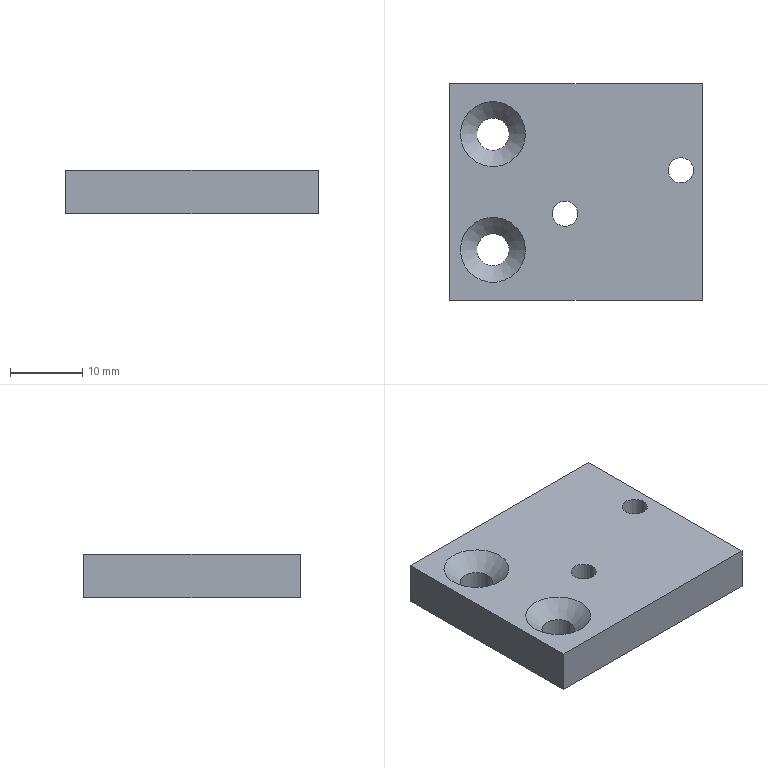Part | NX | 1 solid | 14 faces | box 35 x 30 x 6 mm | volume 5854 mm3 | plane 6 | cylinder 4 | cone 4 | commonest cylinder face diameters 3.5 x2 4.5 x2
STEP:
#1=CARTESIAN_POINT('',(17.5,-15.,0.));
#2=VERTEX_POINT('',#1);
#3=CARTESIAN_POINT('',(17.5,1.197,0.));
#4=VERTEX_POINT('',#3);
#5=CARTESIAN_POINT('',(17.5,-15.,0.));
#6=DIRECTION('',(0.,1.,0.));
#7=VECTOR('',#6,1000.);
#8=LINE('',#5,#7);
#9=EDGE_CURVE('',#2,#4,#8,.T.);
#10=ORIENTED_EDGE('',*,*,#9,.T.);
#11=CARTESIAN_POINT('',(17.5,4.803,0.));
#12=VERTEX_POINT('',#11);
#13=CARTESIAN_POINT('',(17.5,1.197,0.));
#14=CARTESIAN_POINT('',(17.5,1.756,0.2876));
#15=CARTESIAN_POINT('',(17.5,2.993,0.7128));
#16=CARTESIAN_POINT('',(17.5,4.246,0.2868));
#17=CARTESIAN_POINT('',(17.5,4.803,0.));
#18=B_SPLINE_CURVE_WITH_KNOTS('',3,(#13,#14,#15,#16,#17),.UNSPECIFIED.,.F.,.F.,(4,1,4),(0.004834,0.006713,0.008592),.UNSPECIFIED.);
#19=EDGE_CURVE('',#4,#12,#18,.T.);
#20=ORIENTED_EDGE('',*,*,#19,.T.);
#21=CARTESIAN_POINT('',(17.5,15.,0.));
#22=VERTEX_POINT('',#21);
#23=CARTESIAN_POINT('',(17.5,-15.,0.));
#24=DIRECTION('',(0.,1.,0.));
#25=VECTOR('',#24,1000.);
#26=LINE('',#23,#25);
#27=EDGE_CURVE('',#12,#22,#26,.T.);
#28=ORIENTED_EDGE('',*,*,#27,.T.);
#29=CARTESIAN_POINT('',(17.5,15.,6.));
#30=VERTEX_POINT('',#29);
#31=CARTESIAN_POINT('',(17.5,15.,6.));
#32=DIRECTION('',(0.,0.,-1.));
#33=VECTOR('',#32,1000.);
#34=LINE('',#31,#33);
#35=EDGE_CURVE('',#30,#22,#34,.T.);
#36=ORIENTED_EDGE('',*,*,#35,.F.);
#37=CARTESIAN_POINT('',(17.5,-15.,6.));
#38=VERTEX_POINT('',#37);
#39=CARTESIAN_POINT('',(17.5,-15.,6.));
#40=DIRECTION('',(0.,1.,0.));
#41=VECTOR('',#40,1000.);
#42=LINE('',#39,#41);
#43=EDGE_CURVE('',#38,#30,#42,.T.);
#44=ORIENTED_EDGE('',*,*,#43,.F.);
#45=CARTESIAN_POINT('',(17.5,-15.,6.));
#46=DIRECTION('',(0.,0.,-1.));
#47=VECTOR('',#46,1000.);
#48=LINE('',#45,#47);
#49=EDGE_CURVE('',#38,#2,#48,.T.);
#50=ORIENTED_EDGE('',*,*,#49,.T.);
#51=EDGE_LOOP('',(#10,#20,#28,#36,#44,#50));
#52=FACE_BOUND('',#51,.T.);
#53=CARTESIAN_POINT('',(17.5,-15.,6.));
#54=DIRECTION('',(-1.,0.,0.));
#55=DIRECTION('',(0.,0.,1.));
#56=AXIS2_PLACEMENT_3D('',#53,#54,#55);
#57=PLANE('',#56);
#58=ADVANCED_FACE('',(#52),#57,.F.);
#59=CARTESIAN_POINT('',(-17.5,15.,0.));
#60=VERTEX_POINT('',#59);
#61=CARTESIAN_POINT('',(-17.5,15.,0.));
#62=DIRECTION('',(-1.,0.,0.));
#63=VECTOR('',#62,1000.);
#64=LINE('',#61,#63);
#65=EDGE_CURVE('',#22,#60,#64,.T.);
#66=ORIENTED_EDGE('',*,*,#65,.T.);
#67=CARTESIAN_POINT('',(-17.5,15.,6.));
#68=VERTEX_POINT('',#67);
#69=CARTESIAN_POINT('',(-17.5,15.,6.));
#70=DIRECTION('',(0.,0.,-1.));
#71=VECTOR('',#70,1000.);
#72=LINE('',#69,#71);
#73=EDGE_CURVE('',#68,#60,#72,.T.);
#74=ORIENTED_EDGE('',*,*,#73,.F.);
#75=CARTESIAN_POINT('',(-17.5,15.,6.));
#76=DIRECTION('',(-1.,0.,0.));
#77=VECTOR('',#76,1000.);
#78=LINE('',#75,#77);
#79=EDGE_CURVE('',#30,#68,#78,.T.);
#80=ORIENTED_EDGE('',*,*,#79,.F.);
#81=ORIENTED_EDGE('',*,*,#35,.T.);
#82=EDGE_LOOP('',(#66,#74,#80,#81));
#83=FACE_BOUND('',#82,.T.);
#84=CARTESIAN_POINT('',(-17.5,15.,6.));
#85=DIRECTION('',(0.,-1.,0.));
#86=DIRECTION('',(0.,0.,-1.));
#87=AXIS2_PLACEMENT_3D('',#84,#85,#86);
#88=PLANE('',#87);
#89=ADVANCED_FACE('',(#83),#88,.F.);
#90=CARTESIAN_POINT('',(-17.5,-15.,0.));
#91=VERTEX_POINT('',#90);
#92=CARTESIAN_POINT('',(-17.5,-15.,0.));
#93=DIRECTION('',(0.,-1.,0.));
#94=VECTOR('',#93,1000.);
#95=LINE('',#92,#94);
#96=EDGE_CURVE('',#60,#91,#95,.T.);
#97=ORIENTED_EDGE('',*,*,#96,.T.);
#98=CARTESIAN_POINT('',(-17.5,-15.,6.));
#99=VERTEX_POINT('',#98);
#100=CARTESIAN_POINT('',(-17.5,-15.,6.));
#101=DIRECTION('',(0.,0.,-1.));
#102=VECTOR('',#101,1000.);
#103=LINE('',#100,#102);
#104=EDGE_CURVE('',#99,#91,#103,.T.);
#105=ORIENTED_EDGE('',*,*,#104,.F.);
#106=CARTESIAN_POINT('',(-17.5,-15.,6.));
#107=DIRECTION('',(0.,-1.,0.));
#108=VECTOR('',#107,1000.);
#109=LINE('',#106,#108);
#110=EDGE_CURVE('',#68,#99,#109,.T.);
#111=ORIENTED_EDGE('',*,*,#110,.F.);
#112=ORIENTED_EDGE('',*,*,#73,.T.);
#113=EDGE_LOOP('',(#97,#105,#111,#112));
#114=FACE_BOUND('',#113,.T.);
#115=CARTESIAN_POINT('',(-17.5,-15.,6.));
#116=DIRECTION('',(1.,0.,0.));
#117=DIRECTION('',(0.,0.,-1.));
#118=AXIS2_PLACEMENT_3D('',#115,#116,#117);
#119=PLANE('',#118);
#120=ADVANCED_FACE('',(#114),#119,.F.);
#121=CARTESIAN_POINT('',(-17.5,-15.,0.));
#122=DIRECTION('',(1.,0.,0.));
#123=VECTOR('',#122,1000.);
#124=LINE('',#121,#123);
#125=EDGE_CURVE('',#91,#2,#124,.T.);
#126=ORIENTED_EDGE('',*,*,#125,.T.);
#127=ORIENTED_EDGE('',*,*,#49,.F.);
#128=CARTESIAN_POINT('',(-17.5,-15.,6.));
#129=DIRECTION('',(1.,0.,0.));
#130=VECTOR('',#129,1000.);
#131=LINE('',#128,#130);
#132=EDGE_CURVE('',#99,#38,#131,.T.);
#133=ORIENTED_EDGE('',*,*,#132,.F.);
#134=ORIENTED_EDGE('',*,*,#104,.T.);
#135=EDGE_LOOP('',(#126,#127,#133,#134));
#136=FACE_BOUND('',#135,.T.);
#137=CARTESIAN_POINT('',(-17.5,-15.,6.));
#138=DIRECTION('',(0.,1.,0.));
#139=DIRECTION('',(0.,0.,1.));
#140=AXIS2_PLACEMENT_3D('',#137,#138,#139);
#141=PLANE('',#140);
#142=ADVANCED_FACE('',(#136),#141,.F.);
#143=CARTESIAN_POINT('',(-3.25,-3.,6.));
#144=VERTEX_POINT('',#143);
#145=CARTESIAN_POINT('',(-1.5,-3.,6.));
#146=DIRECTION('',(0.,0.,-1.));
#147=DIRECTION('',(-1.,0.,0.));
#148=AXIS2_PLACEMENT_3D('',#145,#146,#147);
#149=CIRCLE('',#148,1.75);
#150=EDGE_CURVE('',#144,#144,#149,.T.);
#151=ORIENTED_EDGE('',*,*,#150,.T.);
#152=EDGE_LOOP('',(#151));
#153=FACE_BOUND('',#152,.T.);
#154=CARTESIAN_POINT('',(12.75,3.,6.));
#155=VERTEX_POINT('',#154);
#156=CARTESIAN_POINT('',(14.5,3.,6.));
#157=DIRECTION('',(0.,0.,-1.));
#158=DIRECTION('',(-1.,0.,0.));
#159=AXIS2_PLACEMENT_3D('',#156,#157,#158);
#160=CIRCLE('',#159,1.75);
#161=EDGE_CURVE('',#155,#155,#160,.T.);
#162=ORIENTED_EDGE('',*,*,#161,.T.);
#163=EDGE_LOOP('',(#162));
#164=FACE_BOUND('',#163,.T.);
#165=CARTESIAN_POINT('',(-7.,8.,6.));
#166=VERTEX_POINT('',#165);
#167=CARTESIAN_POINT('',(-11.5,8.,6.));
#168=DIRECTION('',(0.,0.,1.));
#169=DIRECTION('',(1.,0.,0.));
#170=AXIS2_PLACEMENT_3D('',#167,#168,#169);
#171=CIRCLE('',#170,4.5);
#172=EDGE_CURVE('',#166,#166,#171,.T.);
#173=ORIENTED_EDGE('',*,*,#172,.F.);
#174=EDGE_LOOP('',(#173));
#175=FACE_BOUND('',#174,.T.);
#176=CARTESIAN_POINT('',(-7.,-8.,6.));
#177=VERTEX_POINT('',#176);
#178=CARTESIAN_POINT('',(-11.5,-8.,6.));
#179=DIRECTION('',(0.,0.,1.));
#180=DIRECTION('',(1.,0.,0.));
#181=AXIS2_PLACEMENT_3D('',#178,#179,#180);
#182=CIRCLE('',#181,4.5);
#183=EDGE_CURVE('',#177,#177,#182,.T.);
#184=ORIENTED_EDGE('',*,*,#183,.F.);
#185=EDGE_LOOP('',(#184));
#186=FACE_BOUND('',#185,.T.);
#187=ORIENTED_EDGE('',*,*,#43,.T.);
#188=ORIENTED_EDGE('',*,*,#79,.T.);
#189=ORIENTED_EDGE('',*,*,#110,.T.);
#190=ORIENTED_EDGE('',*,*,#132,.T.);
#191=EDGE_LOOP('',(#187,#188,#189,#190));
#192=FACE_BOUND('',#191,.T.);
#193=CARTESIAN_POINT('',(0.,0.,6.));
#194=DIRECTION('',(0.,0.,-1.));
#195=DIRECTION('',(-1.,0.,0.));
#196=AXIS2_PLACEMENT_3D('',#193,#194,#195);
#197=PLANE('',#196);
#198=ADVANCED_FACE('',(#153,#164,#175,#186,#192),#197,.F.);
#199=CARTESIAN_POINT('',(-5.,-3.,0.));
#200=VERTEX_POINT('',#199);
#201=CARTESIAN_POINT('',(-1.5,-3.,0.));
#202=DIRECTION('',(0.,0.,-1.));
#203=DIRECTION('',(-1.,0.,0.));
#204=AXIS2_PLACEMENT_3D('',#201,#202,#203);
#205=CIRCLE('',#204,3.5);
#206=EDGE_CURVE('',#200,#200,#205,.T.);
#207=ORIENTED_EDGE('',*,*,#206,.F.);
#208=EDGE_LOOP('',(#207));
#209=FACE_BOUND('',#208,.T.);
#210=CARTESIAN_POINT('',(14.5,3.,0.));
#211=DIRECTION('',(0.,0.,-1.));
#212=DIRECTION('',(-1.,0.,0.));
#213=AXIS2_PLACEMENT_3D('',#210,#211,#212);
#214=CIRCLE('',#213,3.5);
#215=EDGE_CURVE('',#4,#12,#214,.T.);
#216=ORIENTED_EDGE('',*,*,#215,.F.);
#217=ORIENTED_EDGE('',*,*,#9,.F.);
#218=ORIENTED_EDGE('',*,*,#125,.F.);
#219=ORIENTED_EDGE('',*,*,#96,.F.);
#220=ORIENTED_EDGE('',*,*,#65,.F.);
#221=ORIENTED_EDGE('',*,*,#27,.F.);
#222=EDGE_LOOP('',(#216,#217,#218,#219,#220,#221));
#223=FACE_BOUND('',#222,.T.);
#224=CARTESIAN_POINT('',(-9.25,8.,0.));
#225=VERTEX_POINT('',#224);
#226=CARTESIAN_POINT('',(-11.5,8.,0.));
#227=DIRECTION('',(0.,0.,1.));
#228=DIRECTION('',(1.,0.,0.));
#229=AXIS2_PLACEMENT_3D('',#226,#227,#228);
#230=CIRCLE('',#229,2.25);
#231=EDGE_CURVE('',#225,#225,#230,.T.);
#232=ORIENTED_EDGE('',*,*,#231,.T.);
#233=EDGE_LOOP('',(#232));
#234=FACE_BOUND('',#233,.T.);
#235=CARTESIAN_POINT('',(-9.25,-8.,0.));
#236=VERTEX_POINT('',#235);
#237=CARTESIAN_POINT('',(-11.5,-8.,0.));
#238=DIRECTION('',(0.,0.,1.));
#239=DIRECTION('',(1.,0.,0.));
#240=AXIS2_PLACEMENT_3D('',#237,#238,#239);
#241=CIRCLE('',#240,2.25);
#242=EDGE_CURVE('',#236,#236,#241,.T.);
#243=ORIENTED_EDGE('',*,*,#242,.T.);
#244=EDGE_LOOP('',(#243));
#245=FACE_BOUND('',#244,.T.);
#246=CARTESIAN_POINT('',(0.,0.,0.));
#247=DIRECTION('',(0.,0.,-1.));
#248=DIRECTION('',(-1.,0.,0.));
#249=AXIS2_PLACEMENT_3D('',#246,#247,#248);
#250=PLANE('',#249);
#251=ADVANCED_FACE('',(#209,#223,#234,#245),#250,.T.);
#252=ORIENTED_EDGE('',*,*,#242,.F.);
#253=EDGE_LOOP('',(#252));
#254=FACE_BOUND('',#253,.T.);
#255=CARTESIAN_POINT('',(-9.25,-8.,3.75));
#256=VERTEX_POINT('',#255);
#257=CARTESIAN_POINT('',(-11.5,-8.,3.75));
#258=DIRECTION('',(0.,0.,1.));
#259=DIRECTION('',(1.,0.,0.));
#260=AXIS2_PLACEMENT_3D('',#257,#258,#259);
#261=CIRCLE('',#260,2.25);
#262=EDGE_CURVE('',#256,#256,#261,.T.);
#263=ORIENTED_EDGE('',*,*,#262,.T.);
#264=EDGE_LOOP('',(#263));
#265=FACE_BOUND('',#264,.T.);
#266=CARTESIAN_POINT('',(-11.5,-8.,6.));
#267=DIRECTION('',(0.,0.,1.));
#268=DIRECTION('',(1.,0.,0.));
#269=AXIS2_PLACEMENT_3D('',#266,#267,#268);
#270=CYLINDRICAL_SURFACE('',#269,2.25);
#271=ADVANCED_FACE('',(#254,#265),#270,.F.);
#272=ORIENTED_EDGE('',*,*,#262,.F.);
#273=EDGE_LOOP('',(#272));
#274=FACE_BOUND('',#273,.T.);
#275=ORIENTED_EDGE('',*,*,#183,.T.);
#276=EDGE_LOOP('',(#275));
#277=FACE_BOUND('',#276,.T.);
#278=CARTESIAN_POINT('',(-11.5,-8.,6.));
#279=DIRECTION('',(0.,0.,1.));
#280=DIRECTION('',(1.,0.,0.));
#281=AXIS2_PLACEMENT_3D('',#278,#279,#280);
#282=CONICAL_SURFACE('',#281,4.5,0.7854);
#283=ADVANCED_FACE('',(#274,#277),#282,.F.);
#284=ORIENTED_EDGE('',*,*,#231,.F.);
#285=EDGE_LOOP('',(#284));
#286=FACE_BOUND('',#285,.T.);
#287=CARTESIAN_POINT('',(-9.25,8.,3.75));
#288=VERTEX_POINT('',#287);
#289=CARTESIAN_POINT('',(-11.5,8.,3.75));
#290=DIRECTION('',(0.,0.,1.));
#291=DIRECTION('',(1.,0.,0.));
#292=AXIS2_PLACEMENT_3D('',#289,#290,#291);
#293=CIRCLE('',#292,2.25);
#294=EDGE_CURVE('',#288,#288,#293,.T.);
#295=ORIENTED_EDGE('',*,*,#294,.T.);
#296=EDGE_LOOP('',(#295));
#297=FACE_BOUND('',#296,.T.);
#298=CARTESIAN_POINT('',(-11.5,8.,6.));
#299=DIRECTION('',(0.,0.,1.));
#300=DIRECTION('',(1.,0.,0.));
#301=AXIS2_PLACEMENT_3D('',#298,#299,#300);
#302=CYLINDRICAL_SURFACE('',#301,2.25);
#303=ADVANCED_FACE('',(#286,#297),#302,.F.);
#304=ORIENTED_EDGE('',*,*,#294,.F.);
#305=EDGE_LOOP('',(#304));
#306=FACE_BOUND('',#305,.T.);
#307=ORIENTED_EDGE('',*,*,#172,.T.);
#308=EDGE_LOOP('',(#307));
#309=FACE_BOUND('',#308,.T.);
#310=CARTESIAN_POINT('',(-11.5,8.,6.));
#311=DIRECTION('',(0.,0.,1.));
#312=DIRECTION('',(1.,0.,0.));
#313=AXIS2_PLACEMENT_3D('',#310,#311,#312);
#314=CONICAL_SURFACE('',#313,4.5,0.7854);
#315=ADVANCED_FACE('',(#306,#309),#314,.F.);
#316=CARTESIAN_POINT('',(12.75,3.,1.75));
#317=VERTEX_POINT('',#316);
#318=CARTESIAN_POINT('',(14.5,3.,1.75));
#319=DIRECTION('',(0.,0.,-1.));
#320=DIRECTION('',(-1.,0.,0.));
#321=AXIS2_PLACEMENT_3D('',#318,#319,#320);
#322=CIRCLE('',#321,1.75);
#323=EDGE_CURVE('',#317,#317,#322,.T.);
#324=ORIENTED_EDGE('',*,*,#323,.F.);
#325=EDGE_LOOP('',(#324));
#326=FACE_BOUND('',#325,.T.);
#327=ORIENTED_EDGE('',*,*,#215,.T.);
#328=ORIENTED_EDGE('',*,*,#19,.F.);
#329=EDGE_LOOP('',(#327,#328));
#330=FACE_BOUND('',#329,.T.);
#331=CARTESIAN_POINT('',(14.5,3.,0.));
#332=DIRECTION('',(0.,0.,-1.));
#333=DIRECTION('',(-1.,0.,0.));
#334=AXIS2_PLACEMENT_3D('',#331,#332,#333);
#335=CONICAL_SURFACE('',#334,3.5,0.7854);
#336=ADVANCED_FACE('',(#326,#330),#335,.F.);
#337=ORIENTED_EDGE('',*,*,#161,.F.);
#338=EDGE_LOOP('',(#337));
#339=FACE_BOUND('',#338,.T.);
#340=ORIENTED_EDGE('',*,*,#323,.T.);
#341=EDGE_LOOP('',(#340));
#342=FACE_BOUND('',#341,.T.);
#343=CARTESIAN_POINT('',(14.5,3.,0.));
#344=DIRECTION('',(0.,0.,-1.));
#345=DIRECTION('',(-1.,0.,0.));
#346=AXIS2_PLACEMENT_3D('',#343,#344,#345);
#347=CYLINDRICAL_SURFACE('',#346,1.75);
#348=ADVANCED_FACE('',(#339,#342),#347,.F.);
#349=ORIENTED_EDGE('',*,*,#150,.F.);
#350=EDGE_LOOP('',(#349));
#351=FACE_BOUND('',#350,.T.);
#352=CARTESIAN_POINT('',(-3.25,-3.,1.75));
#353=VERTEX_POINT('',#352);
#354=CARTESIAN_POINT('',(-1.5,-3.,1.75));
#355=DIRECTION('',(0.,0.,-1.));
#356=DIRECTION('',(-1.,0.,0.));
#357=AXIS2_PLACEMENT_3D('',#354,#355,#356);
#358=CIRCLE('',#357,1.75);
#359=EDGE_CURVE('',#353,#353,#358,.T.);
#360=ORIENTED_EDGE('',*,*,#359,.T.);
#361=EDGE_LOOP('',(#360));
#362=FACE_BOUND('',#361,.T.);
#363=CARTESIAN_POINT('',(-1.5,-3.,0.));
#364=DIRECTION('',(0.,0.,-1.));
#365=DIRECTION('',(-1.,0.,0.));
#366=AXIS2_PLACEMENT_3D('',#363,#364,#365);
#367=CYLINDRICAL_SURFACE('',#366,1.75);
#368=ADVANCED_FACE('',(#351,#362),#367,.F.);
#369=ORIENTED_EDGE('',*,*,#359,.F.);
#370=EDGE_LOOP('',(#369));
#371=FACE_BOUND('',#370,.T.);
#372=ORIENTED_EDGE('',*,*,#206,.T.);
#373=EDGE_LOOP('',(#372));
#374=FACE_BOUND('',#373,.T.);
#375=CARTESIAN_POINT('',(-1.5,-3.,0.));
#376=DIRECTION('',(0.,0.,-1.));
#377=DIRECTION('',(-1.,0.,0.));
#378=AXIS2_PLACEMENT_3D('',#375,#376,#377);
#379=CONICAL_SURFACE('',#378,3.5,0.7854);
#380=ADVANCED_FACE('',(#371,#374),#379,.F.);
#381=CLOSED_SHELL('',(#58,#89,#120,#142,#198,#251,#271,#283,#303,#315,#336,#348,#368,#380));
#382=MANIFOLD_SOLID_BREP('',#381);
#383=(LENGTH_UNIT()NAMED_UNIT(*)SI_UNIT(.MILLI.,.METRE.));
#384=UNCERTAINTY_MEASURE_WITH_UNIT(LENGTH_MEASURE(0.0508),#383,'','');
#385=(NAMED_UNIT(*)PLANE_ANGLE_UNIT()SI_UNIT($,.RADIAN.));
#386=(NAMED_UNIT(*)SI_UNIT($,.STERADIAN.)SOLID_ANGLE_UNIT());
#387=(GEOMETRIC_REPRESENTATION_CONTEXT(3)GLOBAL_UNCERTAINTY_ASSIGNED_CONTEXT((#384))GLOBAL_UNIT_ASSIGNED_CONTEXT((#383,#385,#386))REPRESENTATION_CONTEXT('',''));
#388=ADVANCED_BREP_SHAPE_REPRESENTATION('',(#382),#387);